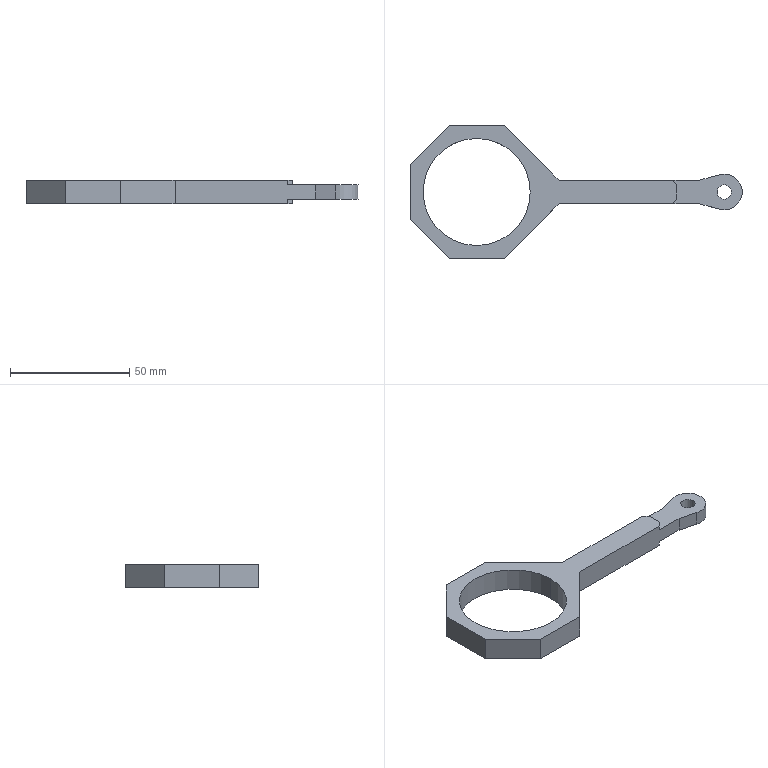Part | SolidWorks | features ICE 2, Extrusion 1 | 1 solid | 26 faces | box 139.5 x 56 x 10 mm | volume 17824 mm3 | plane 21 | cylinder 5 | commonest cylinder face diameters 6 x2 45 x2 15 x1
STEP:
#1=CARTESIAN_POINT('',(101.,0.,-3.));
#2=VERTEX_POINT('',#1);
#3=CARTESIAN_POINT('',(107.,0.,-3.));
#4=VERTEX_POINT('',#3);
#5=CARTESIAN_POINT('',(104.,0.,-3.));
#6=DIRECTION('',(0.,0.,1.));
#7=DIRECTION('',(1.,0.,0.));
#8=AXIS2_PLACEMENT_3D('',#5,#6,#7);
#9=CIRCLE('',#8,3.);
#10=EDGE_CURVE('',#2,#4,#9,.T.);
#11=ORIENTED_EDGE('',*,*,#10,.F.);
#12=CARTESIAN_POINT('',(101.,0.,3.));
#13=VERTEX_POINT('',#12);
#14=CARTESIAN_POINT('',(101.,0.,-12.5));
#15=DIRECTION('',(0.,0.,1.));
#16=VECTOR('',#15,1000.);
#17=LINE('',#14,#16);
#18=EDGE_CURVE('',#2,#13,#17,.T.);
#19=ORIENTED_EDGE('',*,*,#18,.T.);
#20=CARTESIAN_POINT('',(107.,0.,3.));
#21=VERTEX_POINT('',#20);
#22=CARTESIAN_POINT('',(104.,0.,3.));
#23=DIRECTION('',(0.,0.,1.));
#24=DIRECTION('',(1.,0.,0.));
#25=AXIS2_PLACEMENT_3D('',#22,#23,#24);
#26=CIRCLE('',#25,3.);
#27=EDGE_CURVE('',#13,#21,#26,.T.);
#28=ORIENTED_EDGE('',*,*,#27,.T.);
#29=CARTESIAN_POINT('',(107.,0.,-12.5));
#30=DIRECTION('',(0.,0.,1.));
#31=VECTOR('',#30,1000.);
#32=LINE('',#29,#31);
#33=EDGE_CURVE('',#4,#21,#32,.T.);
#34=ORIENTED_EDGE('',*,*,#33,.F.);
#35=EDGE_LOOP('',(#11,#19,#28,#34));
#36=FACE_OUTER_BOUND('',#35,.T.);
#37=CARTESIAN_POINT('',(104.,0.,-12.5));
#38=DIRECTION('',(0.,0.,1.));
#39=DIRECTION('',(1.,0.,0.));
#40=AXIS2_PLACEMENT_3D('',#37,#38,#39);
#41=CYLINDRICAL_SURFACE('',#40,3.);
#42=ADVANCED_FACE('',(#36),#41,.F.);
#43=CARTESIAN_POINT('',(-22.5,0.,5.));
#44=VERTEX_POINT('',#43);
#45=CARTESIAN_POINT('',(22.5,0.,5.));
#46=VERTEX_POINT('',#45);
#47=CARTESIAN_POINT('',(0.,0.,5.));
#48=DIRECTION('',(0.,0.,1.));
#49=DIRECTION('',(1.,0.,0.));
#50=AXIS2_PLACEMENT_3D('',#47,#48,#49);
#51=CIRCLE('',#50,22.5);
#52=EDGE_CURVE('',#44,#46,#51,.T.);
#53=ORIENTED_EDGE('',*,*,#52,.T.);
#54=CARTESIAN_POINT('',(22.5,0.,-5.));
#55=VERTEX_POINT('',#54);
#56=CARTESIAN_POINT('',(22.5,0.,5.));
#57=DIRECTION('',(0.,0.,-1.));
#58=VECTOR('',#57,1000.);
#59=LINE('',#56,#58);
#60=EDGE_CURVE('',#46,#55,#59,.T.);
#61=ORIENTED_EDGE('',*,*,#60,.T.);
#62=CARTESIAN_POINT('',(-22.5,0.,-5.));
#63=VERTEX_POINT('',#62);
#64=CARTESIAN_POINT('',(0.,0.,-5.));
#65=DIRECTION('',(0.,0.,1.));
#66=DIRECTION('',(1.,0.,0.));
#67=AXIS2_PLACEMENT_3D('',#64,#65,#66);
#68=CIRCLE('',#67,22.5);
#69=EDGE_CURVE('',#63,#55,#68,.T.);
#70=ORIENTED_EDGE('',*,*,#69,.F.);
#71=CARTESIAN_POINT('',(-22.5,0.,5.));
#72=DIRECTION('',(0.,0.,-1.));
#73=VECTOR('',#72,1000.);
#74=LINE('',#71,#73);
#75=EDGE_CURVE('',#44,#63,#74,.T.);
#76=ORIENTED_EDGE('',*,*,#75,.F.);
#77=EDGE_LOOP('',(#53,#61,#70,#76));
#78=FACE_OUTER_BOUND('',#77,.T.);
#79=CARTESIAN_POINT('',(0.,0.,5.));
#80=DIRECTION('',(0.,0.,-1.));
#81=DIRECTION('',(-1.,0.,0.));
#82=AXIS2_PLACEMENT_3D('',#79,#80,#81);
#83=CYLINDRICAL_SURFACE('',#82,22.5);
#84=ADVANCED_FACE('',(#78),#83,.F.);
#85=CARTESIAN_POINT('',(84.,-3.,-3.));
#86=VERTEX_POINT('',#85);
#87=CARTESIAN_POINT('',(84.,-3.,-5.));
#88=VERTEX_POINT('',#87);
#89=CARTESIAN_POINT('',(84.,-3.,5.));
#90=DIRECTION('',(0.,0.,-1.));
#91=VECTOR('',#90,1000.);
#92=LINE('',#89,#91);
#93=EDGE_CURVE('',#86,#88,#92,.T.);
#94=ORIENTED_EDGE('',*,*,#93,.F.);
#95=CARTESIAN_POINT('',(82.,-5.,-3.));
#96=VERTEX_POINT('',#95);
#97=CARTESIAN_POINT('',(43.5,-43.5,-3.));
#98=DIRECTION('',(-0.7071,-0.7071,0.));
#99=VECTOR('',#98,1000.);
#100=LINE('',#97,#99);
#101=EDGE_CURVE('',#86,#96,#100,.T.);
#102=ORIENTED_EDGE('',*,*,#101,.T.);
#103=CARTESIAN_POINT('',(82.,-5.,-5.));
#104=VERTEX_POINT('',#103);
#105=CARTESIAN_POINT('',(82.,-5.,5.));
#106=DIRECTION('',(0.,0.,-1.));
#107=VECTOR('',#106,1000.);
#108=LINE('',#105,#107);
#109=EDGE_CURVE('',#96,#104,#108,.T.);
#110=ORIENTED_EDGE('',*,*,#109,.T.);
#111=CARTESIAN_POINT('',(43.5,-43.5,-5.));
#112=DIRECTION('',(-0.7071,-0.7071,0.));
#113=VECTOR('',#112,1000.);
#114=LINE('',#111,#113);
#115=EDGE_CURVE('',#88,#104,#114,.T.);
#116=ORIENTED_EDGE('',*,*,#115,.F.);
#117=EDGE_LOOP('',(#94,#102,#110,#116));
#118=FACE_OUTER_BOUND('',#117,.T.);
#119=CARTESIAN_POINT('',(43.5,-43.5,5.));
#120=DIRECTION('',(0.7071,-0.7071,0.));
#121=DIRECTION('',(0.7071,0.7071,0.));
#122=AXIS2_PLACEMENT_3D('',#119,#120,#121);
#123=PLANE('',#122);
#124=ADVANCED_FACE('',(#118),#123,.T.);
#125=CARTESIAN_POINT('',(84.,3.,-3.));
#126=VERTEX_POINT('',#125);
#127=CARTESIAN_POINT('',(84.,3.,-5.));
#128=VERTEX_POINT('',#127);
#129=CARTESIAN_POINT('',(84.,3.,5.));
#130=DIRECTION('',(0.,0.,-1.));
#131=VECTOR('',#130,1000.);
#132=LINE('',#129,#131);
#133=EDGE_CURVE('',#126,#128,#132,.T.);
#134=ORIENTED_EDGE('',*,*,#133,.F.);
#135=CARTESIAN_POINT('',(84.,0.,-3.));
#136=DIRECTION('',(0.,-1.,0.));
#137=VECTOR('',#136,1000.);
#138=LINE('',#135,#137);
#139=EDGE_CURVE('',#126,#86,#138,.T.);
#140=ORIENTED_EDGE('',*,*,#139,.T.);
#141=ORIENTED_EDGE('',*,*,#93,.T.);
#142=CARTESIAN_POINT('',(84.,0.,-5.));
#143=DIRECTION('',(0.,-1.,0.));
#144=VECTOR('',#143,1000.);
#145=LINE('',#142,#144);
#146=EDGE_CURVE('',#128,#88,#145,.T.);
#147=ORIENTED_EDGE('',*,*,#146,.F.);
#148=EDGE_LOOP('',(#134,#140,#141,#147));
#149=FACE_OUTER_BOUND('',#148,.T.);
#150=CARTESIAN_POINT('',(84.,0.,5.));
#151=DIRECTION('',(1.,0.,0.));
#152=DIRECTION('',(0.,0.,-1.));
#153=AXIS2_PLACEMENT_3D('',#150,#151,#152);
#154=PLANE('',#153);
#155=ADVANCED_FACE('',(#149),#154,.T.);
#156=CARTESIAN_POINT('',(82.,5.,-3.));
#157=VERTEX_POINT('',#156);
#158=CARTESIAN_POINT('',(82.,5.,-5.));
#159=VERTEX_POINT('',#158);
#160=CARTESIAN_POINT('',(82.,5.,5.));
#161=DIRECTION('',(0.,0.,-1.));
#162=VECTOR('',#161,1000.);
#163=LINE('',#160,#162);
#164=EDGE_CURVE('',#157,#159,#163,.T.);
#165=ORIENTED_EDGE('',*,*,#164,.F.);
#166=CARTESIAN_POINT('',(43.5,43.5,-3.));
#167=DIRECTION('',(0.7071,-0.7071,0.));
#168=VECTOR('',#167,1000.);
#169=LINE('',#166,#168);
#170=EDGE_CURVE('',#157,#126,#169,.T.);
#171=ORIENTED_EDGE('',*,*,#170,.T.);
#172=ORIENTED_EDGE('',*,*,#133,.T.);
#173=CARTESIAN_POINT('',(43.5,43.5,-5.));
#174=DIRECTION('',(0.7071,-0.7071,0.));
#175=VECTOR('',#174,1000.);
#176=LINE('',#173,#175);
#177=EDGE_CURVE('',#159,#128,#176,.T.);
#178=ORIENTED_EDGE('',*,*,#177,.F.);
#179=EDGE_LOOP('',(#165,#171,#172,#178));
#180=FACE_OUTER_BOUND('',#179,.T.);
#181=CARTESIAN_POINT('',(43.5,43.5,5.));
#182=DIRECTION('',(0.7071,0.7071,0.));
#183=DIRECTION('',(-0.7071,0.7071,0.));
#184=AXIS2_PLACEMENT_3D('',#181,#182,#183);
#185=PLANE('',#184);
#186=ADVANCED_FACE('',(#180),#185,.T.);
#187=CARTESIAN_POINT('',(84.,-3.,3.));
#188=VERTEX_POINT('',#187);
#189=CARTESIAN_POINT('',(82.,-5.,3.));
#190=VERTEX_POINT('',#189);
#191=CARTESIAN_POINT('',(43.5,-43.5,3.));
#192=DIRECTION('',(-0.7071,-0.7071,0.));
#193=VECTOR('',#192,1000.);
#194=LINE('',#191,#193);
#195=EDGE_CURVE('',#188,#190,#194,.T.);
#196=ORIENTED_EDGE('',*,*,#195,.F.);
#197=CARTESIAN_POINT('',(84.,-3.,5.));
#198=VERTEX_POINT('',#197);
#199=CARTESIAN_POINT('',(84.,-3.,5.));
#200=DIRECTION('',(0.,0.,-1.));
#201=VECTOR('',#200,1000.);
#202=LINE('',#199,#201);
#203=EDGE_CURVE('',#198,#188,#202,.T.);
#204=ORIENTED_EDGE('',*,*,#203,.F.);
#205=CARTESIAN_POINT('',(82.,-5.,5.));
#206=VERTEX_POINT('',#205);
#207=CARTESIAN_POINT('',(43.5,-43.5,5.));
#208=DIRECTION('',(-0.7071,-0.7071,0.));
#209=VECTOR('',#208,1000.);
#210=LINE('',#207,#209);
#211=EDGE_CURVE('',#198,#206,#210,.T.);
#212=ORIENTED_EDGE('',*,*,#211,.T.);
#213=CARTESIAN_POINT('',(82.,-5.,5.));
#214=DIRECTION('',(0.,0.,-1.));
#215=VECTOR('',#214,1000.);
#216=LINE('',#213,#215);
#217=EDGE_CURVE('',#206,#190,#216,.T.);
#218=ORIENTED_EDGE('',*,*,#217,.T.);
#219=EDGE_LOOP('',(#196,#204,#212,#218));
#220=FACE_OUTER_BOUND('',#219,.T.);
#221=CARTESIAN_POINT('',(43.5,-43.5,5.));
#222=DIRECTION('',(0.7071,-0.7071,0.));
#223=DIRECTION('',(0.7071,0.7071,0.));
#224=AXIS2_PLACEMENT_3D('',#221,#222,#223);
#225=PLANE('',#224);
#226=ADVANCED_FACE('',(#220),#225,.T.);
#227=CARTESIAN_POINT('',(84.,3.,3.));
#228=VERTEX_POINT('',#227);
#229=CARTESIAN_POINT('',(84.,0.,3.));
#230=DIRECTION('',(0.,-1.,0.));
#231=VECTOR('',#230,1000.);
#232=LINE('',#229,#231);
#233=EDGE_CURVE('',#228,#188,#232,.T.);
#234=ORIENTED_EDGE('',*,*,#233,.F.);
#235=CARTESIAN_POINT('',(84.,3.,5.));
#236=VERTEX_POINT('',#235);
#237=CARTESIAN_POINT('',(84.,3.,5.));
#238=DIRECTION('',(0.,0.,-1.));
#239=VECTOR('',#238,1000.);
#240=LINE('',#237,#239);
#241=EDGE_CURVE('',#236,#228,#240,.T.);
#242=ORIENTED_EDGE('',*,*,#241,.F.);
#243=CARTESIAN_POINT('',(84.,0.,5.));
#244=DIRECTION('',(0.,-1.,0.));
#245=VECTOR('',#244,1000.);
#246=LINE('',#243,#245);
#247=EDGE_CURVE('',#236,#198,#246,.T.);
#248=ORIENTED_EDGE('',*,*,#247,.T.);
#249=ORIENTED_EDGE('',*,*,#203,.T.);
#250=EDGE_LOOP('',(#234,#242,#248,#249));
#251=FACE_OUTER_BOUND('',#250,.T.);
#252=CARTESIAN_POINT('',(84.,0.,5.));
#253=DIRECTION('',(1.,0.,0.));
#254=DIRECTION('',(0.,0.,-1.));
#255=AXIS2_PLACEMENT_3D('',#252,#253,#254);
#256=PLANE('',#255);
#257=ADVANCED_FACE('',(#251),#256,.T.);
#258=CARTESIAN_POINT('',(82.,5.,3.));
#259=VERTEX_POINT('',#258);
#260=CARTESIAN_POINT('',(43.5,43.5,3.));
#261=DIRECTION('',(0.7071,-0.7071,0.));
#262=VECTOR('',#261,1000.);
#263=LINE('',#260,#262);
#264=EDGE_CURVE('',#259,#228,#263,.T.);
#265=ORIENTED_EDGE('',*,*,#264,.F.);
#266=CARTESIAN_POINT('',(82.,5.,5.));
#267=VERTEX_POINT('',#266);
#268=CARTESIAN_POINT('',(82.,5.,5.));
#269=DIRECTION('',(0.,0.,-1.));
#270=VECTOR('',#269,1000.);
#271=LINE('',#268,#270);
#272=EDGE_CURVE('',#267,#259,#271,.T.);
#273=ORIENTED_EDGE('',*,*,#272,.F.);
#274=CARTESIAN_POINT('',(43.5,43.5,5.));
#275=DIRECTION('',(0.7071,-0.7071,0.));
#276=VECTOR('',#275,1000.);
#277=LINE('',#274,#276);
#278=EDGE_CURVE('',#267,#236,#277,.T.);
#279=ORIENTED_EDGE('',*,*,#278,.T.);
#280=ORIENTED_EDGE('',*,*,#241,.T.);
#281=EDGE_LOOP('',(#265,#273,#279,#280));
#282=FACE_OUTER_BOUND('',#281,.T.);
#283=CARTESIAN_POINT('',(43.5,43.5,5.));
#284=DIRECTION('',(0.7071,0.7071,0.));
#285=DIRECTION('',(-0.7071,0.7071,0.));
#286=AXIS2_PLACEMENT_3D('',#283,#284,#285);
#287=PLANE('',#286);
#288=ADVANCED_FACE('',(#282),#287,.T.);
#289=CARTESIAN_POINT('',(34.598,5.,-5.));
#290=VERTEX_POINT('',#289);
#291=CARTESIAN_POINT('',(0.,5.,-5.));
#292=DIRECTION('',(1.,0.,0.));
#293=VECTOR('',#292,1000.);
#294=LINE('',#291,#293);
#295=EDGE_CURVE('',#290,#159,#294,.T.);
#296=ORIENTED_EDGE('',*,*,#295,.F.);
#297=CARTESIAN_POINT('',(34.598,5.,5.));
#298=VERTEX_POINT('',#297);
#299=CARTESIAN_POINT('',(34.598,5.,5.));
#300=DIRECTION('',(0.,0.,-1.));
#301=VECTOR('',#300,1000.);
#302=LINE('',#299,#301);
#303=EDGE_CURVE('',#298,#290,#302,.T.);
#304=ORIENTED_EDGE('',*,*,#303,.F.);
#305=CARTESIAN_POINT('',(0.,5.,5.));
#306=DIRECTION('',(1.,0.,0.));
#307=VECTOR('',#306,1000.);
#308=LINE('',#305,#307);
#309=EDGE_CURVE('',#298,#267,#308,.T.);
#310=ORIENTED_EDGE('',*,*,#309,.T.);
#311=ORIENTED_EDGE('',*,*,#272,.T.);
#312=CARTESIAN_POINT('',(93.682,5.,3.));
#313=VERTEX_POINT('',#312);
#314=CARTESIAN_POINT('',(0.,5.,3.));
#315=DIRECTION('',(1.,0.,0.));
#316=VECTOR('',#315,1000.);
#317=LINE('',#314,#316);
#318=EDGE_CURVE('',#259,#313,#317,.T.);
#319=ORIENTED_EDGE('',*,*,#318,.T.);
#320=CARTESIAN_POINT('',(93.682,5.,-3.));
#321=VERTEX_POINT('',#320);
#322=CARTESIAN_POINT('',(93.682,5.,3.));
#323=DIRECTION('',(0.,0.,-1.));
#324=VECTOR('',#323,1000.);
#325=LINE('',#322,#324);
#326=EDGE_CURVE('',#313,#321,#325,.T.);
#327=ORIENTED_EDGE('',*,*,#326,.T.);
#328=CARTESIAN_POINT('',(0.,5.,-3.));
#329=DIRECTION('',(1.,0.,0.));
#330=VECTOR('',#329,1000.);
#331=LINE('',#328,#330);
#332=EDGE_CURVE('',#157,#321,#331,.T.);
#333=ORIENTED_EDGE('',*,*,#332,.F.);
#334=ORIENTED_EDGE('',*,*,#164,.T.);
#335=EDGE_LOOP('',(#296,#304,#310,#311,#319,#327,#333,#334));
#336=FACE_OUTER_BOUND('',#335,.T.);
#337=CARTESIAN_POINT('',(0.,5.,5.));
#338=DIRECTION('',(0.,1.,0.));
#339=DIRECTION('',(0.,0.,1.));
#340=AXIS2_PLACEMENT_3D('',#337,#338,#339);
#341=PLANE('',#340);
#342=ADVANCED_FACE('',(#336),#341,.T.);
#343=CARTESIAN_POINT('',(11.598,28.,-5.));
#344=VERTEX_POINT('',#343);
#345=CARTESIAN_POINT('',(19.799,19.799,-5.));
#346=DIRECTION('',(0.7071,-0.7071,0.));
#347=VECTOR('',#346,1000.);
#348=LINE('',#345,#347);
#349=EDGE_CURVE('',#344,#290,#348,.T.);
#350=ORIENTED_EDGE('',*,*,#349,.F.);
#351=CARTESIAN_POINT('',(11.598,28.,5.));
#352=VERTEX_POINT('',#351);
#353=CARTESIAN_POINT('',(11.598,28.,5.));
#354=DIRECTION('',(0.,0.,-1.));
#355=VECTOR('',#354,1000.);
#356=LINE('',#353,#355);
#357=EDGE_CURVE('',#352,#344,#356,.T.);
#358=ORIENTED_EDGE('',*,*,#357,.F.);
#359=CARTESIAN_POINT('',(19.799,19.799,5.));
#360=DIRECTION('',(0.7071,-0.7071,0.));
#361=VECTOR('',#360,1000.);
#362=LINE('',#359,#361);
#363=EDGE_CURVE('',#352,#298,#362,.T.);
#364=ORIENTED_EDGE('',*,*,#363,.T.);
#365=ORIENTED_EDGE('',*,*,#303,.T.);
#366=EDGE_LOOP('',(#350,#358,#364,#365));
#367=FACE_OUTER_BOUND('',#366,.T.);
#368=CARTESIAN_POINT('',(19.799,19.799,5.));
#369=DIRECTION('',(0.7071,0.7071,0.));
#370=DIRECTION('',(-0.7071,0.7071,0.));
#371=AXIS2_PLACEMENT_3D('',#368,#369,#370);
#372=PLANE('',#371);
#373=ADVANCED_FACE('',(#367),#372,.T.);
#374=CARTESIAN_POINT('',(-11.598,28.,-5.));
#375=VERTEX_POINT('',#374);
#376=CARTESIAN_POINT('',(0.,28.,-5.));
#377=DIRECTION('',(-1.,0.,0.));
#378=VECTOR('',#377,1000.);
#379=LINE('',#376,#378);
#380=EDGE_CURVE('',#344,#375,#379,.T.);
#381=ORIENTED_EDGE('',*,*,#380,.T.);
#382=CARTESIAN_POINT('',(-11.598,28.,5.));
#383=VERTEX_POINT('',#382);
#384=CARTESIAN_POINT('',(-11.598,28.,5.));
#385=DIRECTION('',(0.,0.,-1.));
#386=VECTOR('',#385,1000.);
#387=LINE('',#384,#386);
#388=EDGE_CURVE('',#383,#375,#387,.T.);
#389=ORIENTED_EDGE('',*,*,#388,.F.);
#390=CARTESIAN_POINT('',(0.,28.,5.));
#391=DIRECTION('',(-1.,0.,0.));
#392=VECTOR('',#391,1000.);
#393=LINE('',#390,#392);
#394=EDGE_CURVE('',#352,#383,#393,.T.);
#395=ORIENTED_EDGE('',*,*,#394,.F.);
#396=ORIENTED_EDGE('',*,*,#357,.T.);
#397=EDGE_LOOP('',(#381,#389,#395,#396));
#398=FACE_OUTER_BOUND('',#397,.T.);
#399=CARTESIAN_POINT('',(0.,28.,5.));
#400=DIRECTION('',(0.,-1.,0.));
#401=DIRECTION('',(1.,0.,0.));
#402=AXIS2_PLACEMENT_3D('',#399,#400,#401);
#403=PLANE('',#402);
#404=ADVANCED_FACE('',(#398),#403,.F.);
#405=CARTESIAN_POINT('',(-28.,11.598,-5.));
#406=VERTEX_POINT('',#405);
#407=CARTESIAN_POINT('',(-19.799,19.799,-5.));
#408=DIRECTION('',(-0.7071,-0.7071,0.));
#409=VECTOR('',#408,1000.);
#410=LINE('',#407,#409);
#411=EDGE_CURVE('',#375,#406,#410,.T.);
#412=ORIENTED_EDGE('',*,*,#411,.T.);
#413=CARTESIAN_POINT('',(-28.,11.598,5.));
#414=VERTEX_POINT('',#413);
#415=CARTESIAN_POINT('',(-28.,11.598,5.));
#416=DIRECTION('',(0.,0.,-1.));
#417=VECTOR('',#416,1000.);
#418=LINE('',#415,#417);
#419=EDGE_CURVE('',#414,#406,#418,.T.);
#420=ORIENTED_EDGE('',*,*,#419,.F.);
#421=CARTESIAN_POINT('',(-19.799,19.799,5.));
#422=DIRECTION('',(-0.7071,-0.7071,0.));
#423=VECTOR('',#422,1000.);
#424=LINE('',#421,#423);
#425=EDGE_CURVE('',#383,#414,#424,.T.);
#426=ORIENTED_EDGE('',*,*,#425,.F.);
#427=ORIENTED_EDGE('',*,*,#388,.T.);
#428=EDGE_LOOP('',(#412,#420,#426,#427));
#429=FACE_OUTER_BOUND('',#428,.T.);
#430=CARTESIAN_POINT('',(-19.799,19.799,5.));
#431=DIRECTION('',(0.7071,-0.7071,0.));
#432=DIRECTION('',(0.7071,0.7071,0.));
#433=AXIS2_PLACEMENT_3D('',#430,#431,#432);
#434=PLANE('',#433);
#435=ADVANCED_FACE('',(#429),#434,.F.);
#436=CARTESIAN_POINT('',(-28.,-11.598,-5.));
#437=VERTEX_POINT('',#436);
#438=CARTESIAN_POINT('',(-28.,0.,-5.));
#439=DIRECTION('',(0.,-1.,0.));
#440=VECTOR('',#439,1000.);
#441=LINE('',#438,#440);
#442=EDGE_CURVE('',#406,#437,#441,.T.);
#443=ORIENTED_EDGE('',*,*,#442,.T.);
#444=CARTESIAN_POINT('',(-28.,-11.598,5.));
#445=VERTEX_POINT('',#444);
#446=CARTESIAN_POINT('',(-28.,-11.598,5.));
#447=DIRECTION('',(0.,0.,-1.));
#448=VECTOR('',#447,1000.);
#449=LINE('',#446,#448);
#450=EDGE_CURVE('',#445,#437,#449,.T.);
#451=ORIENTED_EDGE('',*,*,#450,.F.);
#452=CARTESIAN_POINT('',(-28.,0.,5.));
#453=DIRECTION('',(0.,-1.,0.));
#454=VECTOR('',#453,1000.);
#455=LINE('',#452,#454);
#456=EDGE_CURVE('',#414,#445,#455,.T.);
#457=ORIENTED_EDGE('',*,*,#456,.F.);
#458=ORIENTED_EDGE('',*,*,#419,.T.);
#459=EDGE_LOOP('',(#443,#451,#457,#458));
#460=FACE_OUTER_BOUND('',#459,.T.);
#461=CARTESIAN_POINT('',(-28.,0.,5.));
#462=DIRECTION('',(1.,0.,0.));
#463=DIRECTION('',(0.,1.,0.));
#464=AXIS2_PLACEMENT_3D('',#461,#462,#463);
#465=PLANE('',#464);
#466=ADVANCED_FACE('',(#460),#465,.F.);
#467=CARTESIAN_POINT('',(-11.598,-28.,-5.));
#468=VERTEX_POINT('',#467);
#469=CARTESIAN_POINT('',(-19.799,-19.799,-5.));
#470=DIRECTION('',(0.7071,-0.7071,0.));
#471=VECTOR('',#470,1000.);
#472=LINE('',#469,#471);
#473=EDGE_CURVE('',#437,#468,#472,.T.);
#474=ORIENTED_EDGE('',*,*,#473,.T.);
#475=CARTESIAN_POINT('',(-11.598,-28.,5.));
#476=VERTEX_POINT('',#475);
#477=CARTESIAN_POINT('',(-11.598,-28.,5.));
#478=DIRECTION('',(0.,0.,-1.));
#479=VECTOR('',#478,1000.);
#480=LINE('',#477,#479);
#481=EDGE_CURVE('',#476,#468,#480,.T.);
#482=ORIENTED_EDGE('',*,*,#481,.F.);
#483=CARTESIAN_POINT('',(-19.799,-19.799,5.));
#484=DIRECTION('',(0.7071,-0.7071,0.));
#485=VECTOR('',#484,1000.);
#486=LINE('',#483,#485);
#487=EDGE_CURVE('',#445,#476,#486,.T.);
#488=ORIENTED_EDGE('',*,*,#487,.F.);
#489=ORIENTED_EDGE('',*,*,#450,.T.);
#490=EDGE_LOOP('',(#474,#482,#488,#489));
#491=FACE_OUTER_BOUND('',#490,.T.);
#492=CARTESIAN_POINT('',(-19.799,-19.799,5.));
#493=DIRECTION('',(0.7071,0.7071,0.));
#494=DIRECTION('',(-0.7071,0.7071,0.));
#495=AXIS2_PLACEMENT_3D('',#492,#493,#494);
#496=PLANE('',#495);
#497=ADVANCED_FACE('',(#491),#496,.F.);
#498=CARTESIAN_POINT('',(11.598,-28.,-5.));
#499=VERTEX_POINT('',#498);
#500=CARTESIAN_POINT('',(0.,-28.,-5.));
#501=DIRECTION('',(1.,0.,0.));
#502=VECTOR('',#501,1000.);
#503=LINE('',#500,#502);
#504=EDGE_CURVE('',#468,#499,#503,.T.);
#505=ORIENTED_EDGE('',*,*,#504,.T.);
#506=CARTESIAN_POINT('',(11.598,-28.,5.));
#507=VERTEX_POINT('',#506);
#508=CARTESIAN_POINT('',(11.598,-28.,5.));
#509=DIRECTION('',(0.,0.,-1.));
#510=VECTOR('',#509,1000.);
#511=LINE('',#508,#510);
#512=EDGE_CURVE('',#507,#499,#511,.T.);
#513=ORIENTED_EDGE('',*,*,#512,.F.);
#514=CARTESIAN_POINT('',(0.,-28.,5.));
#515=DIRECTION('',(1.,0.,0.));
#516=VECTOR('',#515,1000.);
#517=LINE('',#514,#516);
#518=EDGE_CURVE('',#476,#507,#517,.T.);
#519=ORIENTED_EDGE('',*,*,#518,.F.);
#520=ORIENTED_EDGE('',*,*,#481,.T.);
#521=EDGE_LOOP('',(#505,#513,#519,#520));
#522=FACE_OUTER_BOUND('',#521,.T.);
#523=CARTESIAN_POINT('',(0.,-28.,5.));
#524=DIRECTION('',(0.,1.,0.));
#525=DIRECTION('',(-1.,0.,0.));
#526=AXIS2_PLACEMENT_3D('',#523,#524,#525);
#527=PLANE('',#526);
#528=ADVANCED_FACE('',(#522),#527,.F.);
#529=CARTESIAN_POINT('',(34.598,-5.,-5.));
#530=VERTEX_POINT('',#529);
#531=CARTESIAN_POINT('',(19.799,-19.799,-5.));
#532=DIRECTION('',(0.7071,0.7071,0.));
#533=VECTOR('',#532,1000.);
#534=LINE('',#531,#533);
#535=EDGE_CURVE('',#499,#530,#534,.T.);
#536=ORIENTED_EDGE('',*,*,#535,.T.);
#537=CARTESIAN_POINT('',(34.598,-5.,5.));
#538=VERTEX_POINT('',#537);
#539=CARTESIAN_POINT('',(34.598,-5.,5.));
#540=DIRECTION('',(0.,0.,-1.));
#541=VECTOR('',#540,1000.);
#542=LINE('',#539,#541);
#543=EDGE_CURVE('',#538,#530,#542,.T.);
#544=ORIENTED_EDGE('',*,*,#543,.F.);
#545=CARTESIAN_POINT('',(19.799,-19.799,5.));
#546=DIRECTION('',(0.7071,0.7071,0.));
#547=VECTOR('',#546,1000.);
#548=LINE('',#545,#547);
#549=EDGE_CURVE('',#507,#538,#548,.T.);
#550=ORIENTED_EDGE('',*,*,#549,.F.);
#551=ORIENTED_EDGE('',*,*,#512,.T.);
#552=EDGE_LOOP('',(#536,#544,#550,#551));
#553=FACE_OUTER_BOUND('',#552,.T.);
#554=CARTESIAN_POINT('',(19.799,-19.799,5.));
#555=DIRECTION('',(-0.7071,0.7071,0.));
#556=DIRECTION('',(-0.7071,-0.7071,0.));
#557=AXIS2_PLACEMENT_3D('',#554,#555,#556);
#558=PLANE('',#557);
#559=ADVANCED_FACE('',(#553),#558,.F.);
#560=ORIENTED_EDGE('',*,*,#60,.F.);
#561=CARTESIAN_POINT('',(0.,0.,5.));
#562=DIRECTION('',(0.,0.,1.));
#563=DIRECTION('',(1.,0.,0.));
#564=AXIS2_PLACEMENT_3D('',#561,#562,#563);
#565=CIRCLE('',#564,22.5);
#566=EDGE_CURVE('',#46,#44,#565,.T.);
#567=ORIENTED_EDGE('',*,*,#566,.T.);
#568=ORIENTED_EDGE('',*,*,#75,.T.);
#569=CARTESIAN_POINT('',(0.,0.,-5.));
#570=DIRECTION('',(0.,0.,1.));
#571=DIRECTION('',(1.,0.,0.));
#572=AXIS2_PLACEMENT_3D('',#569,#570,#571);
#573=CIRCLE('',#572,22.5);
#574=EDGE_CURVE('',#55,#63,#573,.T.);
#575=ORIENTED_EDGE('',*,*,#574,.F.);
#576=EDGE_LOOP('',(#560,#567,#568,#575));
#577=FACE_OUTER_BOUND('',#576,.T.);
#578=CARTESIAN_POINT('',(0.,0.,5.));
#579=DIRECTION('',(0.,0.,-1.));
#580=DIRECTION('',(-1.,0.,0.));
#581=AXIS2_PLACEMENT_3D('',#578,#579,#580);
#582=CYLINDRICAL_SURFACE('',#581,22.5);
#583=ADVANCED_FACE('',(#577),#582,.F.);
#584=CARTESIAN_POINT('',(0.,-5.,-5.));
#585=DIRECTION('',(1.,0.,0.));
#586=VECTOR('',#585,1000.);
#587=LINE('',#584,#586);
#588=EDGE_CURVE('',#530,#104,#587,.T.);
#589=ORIENTED_EDGE('',*,*,#588,.T.);
#590=ORIENTED_EDGE('',*,*,#109,.F.);
#591=CARTESIAN_POINT('',(93.682,-5.,-3.));
#592=VERTEX_POINT('',#591);
#593=CARTESIAN_POINT('',(0.,-5.,-3.));
#594=DIRECTION('',(1.,0.,0.));
#595=VECTOR('',#594,1000.);
#596=LINE('',#593,#595);
#597=EDGE_CURVE('',#96,#592,#596,.T.);
#598=ORIENTED_EDGE('',*,*,#597,.T.);
#599=CARTESIAN_POINT('',(93.682,-5.,3.));
#600=VERTEX_POINT('',#599);
#601=CARTESIAN_POINT('',(93.682,-5.,3.));
#602=DIRECTION('',(0.,0.,-1.));
#603=VECTOR('',#602,1000.);
#604=LINE('',#601,#603);
#605=EDGE_CURVE('',#600,#592,#604,.T.);
#606=ORIENTED_EDGE('',*,*,#605,.F.);
#607=CARTESIAN_POINT('',(0.,-5.,3.));
#608=DIRECTION('',(1.,0.,0.));
#609=VECTOR('',#608,1000.);
#610=LINE('',#607,#609);
#611=EDGE_CURVE('',#190,#600,#610,.T.);
#612=ORIENTED_EDGE('',*,*,#611,.F.);
#613=ORIENTED_EDGE('',*,*,#217,.F.);
#614=CARTESIAN_POINT('',(0.,-5.,5.));
#615=DIRECTION('',(1.,0.,0.));
#616=VECTOR('',#615,1000.);
#617=LINE('',#614,#616);
#618=EDGE_CURVE('',#538,#206,#617,.T.);
#619=ORIENTED_EDGE('',*,*,#618,.F.);
#620=ORIENTED_EDGE('',*,*,#543,.T.);
#621=EDGE_LOOP('',(#589,#590,#598,#606,#612,#613,#619,#620));
#622=FACE_OUTER_BOUND('',#621,.T.);
#623=CARTESIAN_POINT('',(0.,-5.,5.));
#624=DIRECTION('',(0.,1.,0.));
#625=DIRECTION('',(-1.,0.,0.));
#626=AXIS2_PLACEMENT_3D('',#623,#624,#625);
#627=PLANE('',#626);
#628=ADVANCED_FACE('',(#622),#627,.F.);
#629=ORIENTED_EDGE('',*,*,#52,.F.);
#630=ORIENTED_EDGE('',*,*,#566,.F.);
#631=EDGE_LOOP('',(#629,#630));
#632=FACE_BOUND('',#631,.T.);
#633=ORIENTED_EDGE('',*,*,#211,.F.);
#634=ORIENTED_EDGE('',*,*,#247,.F.);
#635=ORIENTED_EDGE('',*,*,#278,.F.);
#636=ORIENTED_EDGE('',*,*,#309,.F.);
#637=ORIENTED_EDGE('',*,*,#363,.F.);
#638=ORIENTED_EDGE('',*,*,#394,.T.);
#639=ORIENTED_EDGE('',*,*,#425,.T.);
#640=ORIENTED_EDGE('',*,*,#456,.T.);
#641=ORIENTED_EDGE('',*,*,#487,.T.);
#642=ORIENTED_EDGE('',*,*,#518,.T.);
#643=ORIENTED_EDGE('',*,*,#549,.T.);
#644=ORIENTED_EDGE('',*,*,#618,.T.);
#645=EDGE_LOOP('',(#633,#634,#635,#636,#637,#638,#639,#640,#641,#642,#643,#644));
#646=FACE_OUTER_BOUND('',#645,.T.);
#647=CARTESIAN_POINT('',(0.,0.,5.));
#648=DIRECTION('',(0.,0.,1.));
#649=DIRECTION('',(1.,0.,0.));
#650=AXIS2_PLACEMENT_3D('',#647,#648,#649);
#651=PLANE('',#650);
#652=ADVANCED_FACE('',(#632,#646),#651,.T.);
#653=ORIENTED_EDGE('',*,*,#69,.T.);
#654=ORIENTED_EDGE('',*,*,#574,.T.);
#655=EDGE_LOOP('',(#653,#654));
#656=FACE_BOUND('',#655,.T.);
#657=ORIENTED_EDGE('',*,*,#115,.T.);
#658=ORIENTED_EDGE('',*,*,#588,.F.);
#659=ORIENTED_EDGE('',*,*,#535,.F.);
#660=ORIENTED_EDGE('',*,*,#504,.F.);
#661=ORIENTED_EDGE('',*,*,#473,.F.);
#662=ORIENTED_EDGE('',*,*,#442,.F.);
#663=ORIENTED_EDGE('',*,*,#411,.F.);
#664=ORIENTED_EDGE('',*,*,#380,.F.);
#665=ORIENTED_EDGE('',*,*,#349,.T.);
#666=ORIENTED_EDGE('',*,*,#295,.T.);
#667=ORIENTED_EDGE('',*,*,#177,.T.);
#668=ORIENTED_EDGE('',*,*,#146,.T.);
#669=EDGE_LOOP('',(#657,#658,#659,#660,#661,#662,#663,#664,#665,#666,#667,#668));
#670=FACE_OUTER_BOUND('',#669,.T.);
#671=CARTESIAN_POINT('',(0.,0.,-5.));
#672=DIRECTION('',(0.,0.,1.));
#673=DIRECTION('',(1.,0.,0.));
#674=AXIS2_PLACEMENT_3D('',#671,#672,#673);
#675=PLANE('',#674);
#676=ADVANCED_FACE('',(#656,#670),#675,.F.);
#677=CARTESIAN_POINT('',(102.059,-7.244,-3.));
#678=VERTEX_POINT('',#677);
#679=CARTESIAN_POINT('',(5.026,18.756,-3.));
#680=DIRECTION('',(0.9659,-0.2588,0.));
#681=VECTOR('',#680,1000.);
#682=LINE('',#679,#681);
#683=EDGE_CURVE('',#592,#678,#682,.T.);
#684=ORIENTED_EDGE('',*,*,#683,.T.);
#685=CARTESIAN_POINT('',(102.059,-7.244,3.));
#686=VERTEX_POINT('',#685);
#687=CARTESIAN_POINT('',(102.059,-7.244,3.));
#688=DIRECTION('',(0.,0.,-1.));
#689=VECTOR('',#688,1000.);
#690=LINE('',#687,#689);
#691=EDGE_CURVE('',#686,#678,#690,.T.);
#692=ORIENTED_EDGE('',*,*,#691,.F.);
#693=CARTESIAN_POINT('',(5.026,18.756,3.));
#694=DIRECTION('',(0.9659,-0.2588,0.));
#695=VECTOR('',#694,1000.);
#696=LINE('',#693,#695);
#697=EDGE_CURVE('',#600,#686,#696,.T.);
#698=ORIENTED_EDGE('',*,*,#697,.F.);
#699=ORIENTED_EDGE('',*,*,#605,.T.);
#700=EDGE_LOOP('',(#684,#692,#698,#699));
#701=FACE_OUTER_BOUND('',#700,.T.);
#702=CARTESIAN_POINT('',(5.026,18.756,3.));
#703=DIRECTION('',(0.2588,0.9659,0.));
#704=DIRECTION('',(-0.9659,0.2588,0.));
#705=AXIS2_PLACEMENT_3D('',#702,#703,#704);
#706=PLANE('',#705);
#707=ADVANCED_FACE('',(#701),#706,.F.);
#708=CARTESIAN_POINT('',(102.059,7.244,-3.));
#709=VERTEX_POINT('',#708);
#710=CARTESIAN_POINT('',(104.,0.,-3.));
#711=DIRECTION('',(0.,0.,1.));
#712=DIRECTION('',(1.,0.,0.));
#713=AXIS2_PLACEMENT_3D('',#710,#711,#712);
#714=CIRCLE('',#713,7.5);
#715=EDGE_CURVE('',#678,#709,#714,.T.);
#716=ORIENTED_EDGE('',*,*,#715,.T.);
#717=CARTESIAN_POINT('',(102.059,7.244,3.));
#718=VERTEX_POINT('',#717);
#719=CARTESIAN_POINT('',(102.059,7.244,3.));
#720=DIRECTION('',(0.,0.,-1.));
#721=VECTOR('',#720,1000.);
#722=LINE('',#719,#721);
#723=EDGE_CURVE('',#718,#709,#722,.T.);
#724=ORIENTED_EDGE('',*,*,#723,.F.);
#725=CARTESIAN_POINT('',(104.,0.,3.));
#726=DIRECTION('',(0.,0.,1.));
#727=DIRECTION('',(1.,0.,0.));
#728=AXIS2_PLACEMENT_3D('',#725,#726,#727);
#729=CIRCLE('',#728,7.5);
#730=EDGE_CURVE('',#686,#718,#729,.T.);
#731=ORIENTED_EDGE('',*,*,#730,.F.);
#732=ORIENTED_EDGE('',*,*,#691,.T.);
#733=EDGE_LOOP('',(#716,#724,#731,#732));
#734=FACE_OUTER_BOUND('',#733,.T.);
#735=CARTESIAN_POINT('',(104.,0.,3.));
#736=DIRECTION('',(0.,0.,-1.));
#737=DIRECTION('',(-1.,0.,0.));
#738=AXIS2_PLACEMENT_3D('',#735,#736,#737);
#739=CYLINDRICAL_SURFACE('',#738,7.5);
#740=ADVANCED_FACE('',(#734),#739,.T.);
#741=CARTESIAN_POINT('',(5.026,-18.756,-3.));
#742=DIRECTION('',(0.9659,0.2588,0.));
#743=VECTOR('',#742,1000.);
#744=LINE('',#741,#743);
#745=EDGE_CURVE('',#321,#709,#744,.T.);
#746=ORIENTED_EDGE('',*,*,#745,.F.);
#747=ORIENTED_EDGE('',*,*,#326,.F.);
#748=CARTESIAN_POINT('',(5.026,-18.756,3.));
#749=DIRECTION('',(0.9659,0.2588,0.));
#750=VECTOR('',#749,1000.);
#751=LINE('',#748,#750);
#752=EDGE_CURVE('',#313,#718,#751,.T.);
#753=ORIENTED_EDGE('',*,*,#752,.T.);
#754=ORIENTED_EDGE('',*,*,#723,.T.);
#755=EDGE_LOOP('',(#746,#747,#753,#754));
#756=FACE_OUTER_BOUND('',#755,.T.);
#757=CARTESIAN_POINT('',(5.026,-18.756,3.));
#758=DIRECTION('',(-0.2588,0.9659,0.));
#759=DIRECTION('',(-0.9659,-0.2588,0.));
#760=AXIS2_PLACEMENT_3D('',#757,#758,#759);
#761=PLANE('',#760);
#762=ADVANCED_FACE('',(#756),#761,.T.);
#763=CARTESIAN_POINT('',(104.,0.,3.));
#764=DIRECTION('',(0.,0.,1.));
#765=DIRECTION('',(1.,0.,0.));
#766=AXIS2_PLACEMENT_3D('',#763,#764,#765);
#767=CIRCLE('',#766,3.);
#768=EDGE_CURVE('',#21,#13,#767,.T.);
#769=ORIENTED_EDGE('',*,*,#768,.F.);
#770=ORIENTED_EDGE('',*,*,#27,.F.);
#771=EDGE_LOOP('',(#769,#770));
#772=FACE_BOUND('',#771,.T.);
#773=ORIENTED_EDGE('',*,*,#697,.T.);
#774=ORIENTED_EDGE('',*,*,#730,.T.);
#775=ORIENTED_EDGE('',*,*,#752,.F.);
#776=ORIENTED_EDGE('',*,*,#318,.F.);
#777=ORIENTED_EDGE('',*,*,#264,.T.);
#778=ORIENTED_EDGE('',*,*,#233,.T.);
#779=ORIENTED_EDGE('',*,*,#195,.T.);
#780=ORIENTED_EDGE('',*,*,#611,.T.);
#781=EDGE_LOOP('',(#773,#774,#775,#776,#777,#778,#779,#780));
#782=FACE_OUTER_BOUND('',#781,.T.);
#783=CARTESIAN_POINT('',(0.,0.,3.));
#784=DIRECTION('',(0.,0.,1.));
#785=DIRECTION('',(1.,0.,0.));
#786=AXIS2_PLACEMENT_3D('',#783,#784,#785);
#787=PLANE('',#786);
#788=ADVANCED_FACE('',(#772,#782),#787,.T.);
#789=CARTESIAN_POINT('',(104.,0.,-3.));
#790=DIRECTION('',(0.,0.,1.));
#791=DIRECTION('',(1.,0.,0.));
#792=AXIS2_PLACEMENT_3D('',#789,#790,#791);
#793=CIRCLE('',#792,3.);
#794=EDGE_CURVE('',#4,#2,#793,.T.);
#795=ORIENTED_EDGE('',*,*,#794,.T.);
#796=ORIENTED_EDGE('',*,*,#10,.T.);
#797=EDGE_LOOP('',(#795,#796));
#798=FACE_BOUND('',#797,.T.);
#799=ORIENTED_EDGE('',*,*,#683,.F.);
#800=ORIENTED_EDGE('',*,*,#597,.F.);
#801=ORIENTED_EDGE('',*,*,#101,.F.);
#802=ORIENTED_EDGE('',*,*,#139,.F.);
#803=ORIENTED_EDGE('',*,*,#170,.F.);
#804=ORIENTED_EDGE('',*,*,#332,.T.);
#805=ORIENTED_EDGE('',*,*,#745,.T.);
#806=ORIENTED_EDGE('',*,*,#715,.F.);
#807=EDGE_LOOP('',(#799,#800,#801,#802,#803,#804,#805,#806));
#808=FACE_OUTER_BOUND('',#807,.T.);
#809=CARTESIAN_POINT('',(0.,0.,-3.));
#810=DIRECTION('',(0.,0.,1.));
#811=DIRECTION('',(1.,0.,0.));
#812=AXIS2_PLACEMENT_3D('',#809,#810,#811);
#813=PLANE('',#812);
#814=ADVANCED_FACE('',(#798,#808),#813,.F.);
#815=ORIENTED_EDGE('',*,*,#18,.F.);
#816=ORIENTED_EDGE('',*,*,#794,.F.);
#817=ORIENTED_EDGE('',*,*,#33,.T.);
#818=ORIENTED_EDGE('',*,*,#768,.T.);
#819=EDGE_LOOP('',(#815,#816,#817,#818));
#820=FACE_OUTER_BOUND('',#819,.T.);
#821=CARTESIAN_POINT('',(104.,0.,-12.5));
#822=DIRECTION('',(0.,0.,1.));
#823=DIRECTION('',(1.,0.,0.));
#824=AXIS2_PLACEMENT_3D('',#821,#822,#823);
#825=CYLINDRICAL_SURFACE('',#824,3.);
#826=ADVANCED_FACE('',(#820),#825,.F.);
#827=CLOSED_SHELL('',(#42,#84,#124,#155,#186,#226,#257,#288,#342,#373,#404,#435,#466,#497,#528,#559,#583,#628,#652,#676,#707,#740,#762,#788,#814,#826));
#828=MANIFOLD_SOLID_BREP('',#827);
#829=CARTESIAN_POINT('',(0.,0.,0.));
#830=DIRECTION('',(0.,0.,1.));
#831=DIRECTION('',(1.,0.,0.));
#832=AXIS2_PLACEMENT_3D('',#829,#830,#831);
#833=(LENGTH_UNIT()NAMED_UNIT(*)SI_UNIT(.MILLI.,.METRE.));
#834=UNCERTAINTY_MEASURE_WITH_UNIT(LENGTH_MEASURE(0.00001),#833,'','');
#835=(NAMED_UNIT(*)PLANE_ANGLE_UNIT()SI_UNIT($,.RADIAN.));
#836=(NAMED_UNIT(*)SI_UNIT($,.STERADIAN.)SOLID_ANGLE_UNIT());
#837=(GEOMETRIC_REPRESENTATION_CONTEXT(3)GLOBAL_UNCERTAINTY_ASSIGNED_CONTEXT((#834))GLOBAL_UNIT_ASSIGNED_CONTEXT((#833,#835,#836))REPRESENTATION_CONTEXT('',''));
#838=ADVANCED_BREP_SHAPE_REPRESENTATION('',(#828,#832),#837);